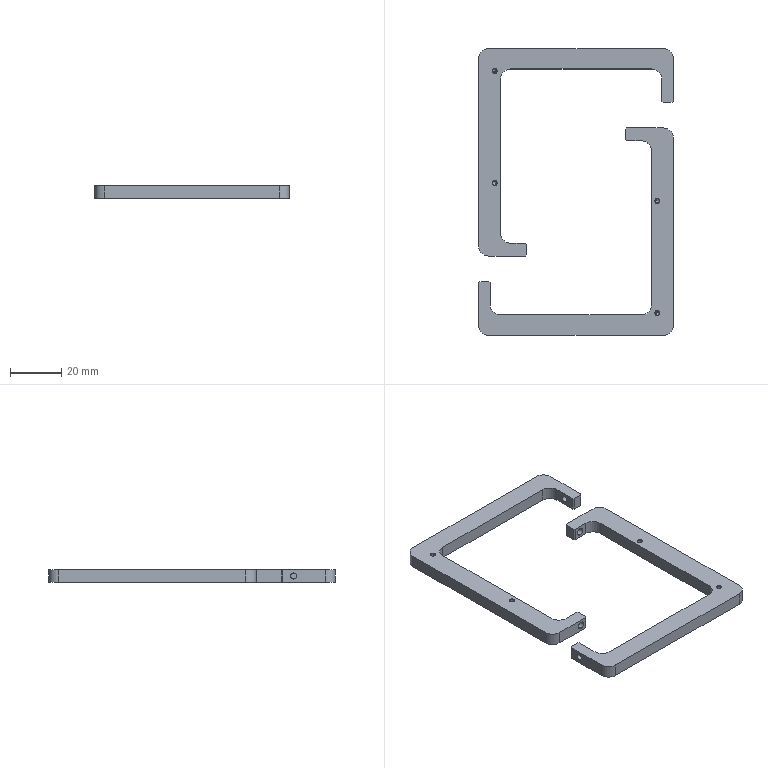CAM job | NX | 3+2 milling, drilling | part box 76 x 112 x 5 mm | stock box 76 x 112 x 5 mm
Tools:
number,name,description,diameter,corner_radius,flute_length,length,flutes
3,CHAMFER_D4-90DEG,倒角D4-90度,4.0,0.0,5.0,50.0,2
5,DRILL_D1.84-11-D3-40,钻刀D1.84-11-D3-40,1.84,0.0,11.0,12.0,2
10,DRILL_D2.4-11-D3-40,钻刀D1.84-11-D3-40,2.4,0.0,11.0,12.0,2
10,DRILL_D2.9-11-D3-40,钻刀D1.84-11-D3-40,2.9,0.0,11.0,12.0,2
6,FORM_M2-12-D3-39,挤压M2-12-D3-39,2.0,0.0,12.5,14.5,2
1,D4_ROUGH,Milling Tool-5 Parameters,4.0,0.0,50.0,75.0,2
2,D4-16-D4-75-3T,D4-16-D4-75-3T,4.0,0.0,16.0,75.0,3
1,CHAMFER_D3-90DEG,倒角D3-90度,3.0,0.0,5.0,50.0,2
Operations:
program,operation,operation_type,tool,method,geometry_group,spindle_rpm,surface_speed,feed_per_tooth,feed_cut,feed_plunge,cut_length_mm,path_length_mm,cut_time_min,machine_time_min
B1,DRILLING_1,Operation,CHAMFER_D4-90DEG,METHOD,WORKPIECE,3000.0,37.0,0.0333,200.0,0.0,16.2,250.449,0.081,0.1044
B2,DRILLING_1_COPY,Operation,DRILL_D1.84-11-D3-40,METHOD,WORKPIECE,3000.0,17.0,0.0167,100.0,0.0,30.4,278.849,0.304,0.3288
B3,DRILLING_1_COPY_COPY,Operation,FORM_M2-12-D3-39,METHOD,WORKPIECE,300.0,1.0,0.2,120.0,0.0,29.2,276.449,0.2433,0.2681
B4,FLOOR_WALL_1,VolumeBased25DMillingOperation,D4_ROUGH,METHOD,WORKPIECE,6500.0,81.0,0.1538,2000.0,100.0,2667.244,2912.294,1.334,1.358
B4,FLOOR_WALL_1_COPY,VolumeBased25DMillingOperation,D4-16-D4-75-3T,METHOD,WORKPIECE,6500.0,81.0,0.041,800.0,100.0,1333.622,1475.488,1.667,1.681
B5,PLANAR_MILL_2,PlanarMilling,D4_ROUGH,METHOD,WORKPIECE,6500.0,81.0,0.1154,1500.0,100.0,10303.227,10451.343,6.869,6.884
B5,PLANAR_MILL_2_COPY,PlanarMilling,D4-16-D4-75-3T,METHOD,WORKPIECE,6500.0,81.0,0.041,800.0,100.0,736.644,887.18,0.9208,0.9359
B6,PLANAR_MILL_1_COPY,PlanarMilling,CHAMFER_D3-90DEG,METHOD,WORKPIECE,6500.0,100.0,0.1178,1200.0,100.0,729.278,888.008,0.6077,0.6236
G55,DRILLING,Operation,CHAMFER_D4-90DEG,METHOD,G55,1200.0,15.0,0.0417,100.0,0.0,4.2,48.4,0.042,0.0464
G55,DRILLING_COPY,Operation,DRILL_D2.4-11-D3-40,METHOD,G55,2000.0,15.0,0.025,100.0,0.0,9.0,58.0,0.09,0.0949
G56,DRILLING_COPY_1,Operation,CHAMFER_D4-90DEG,METHOD,G56,1200.0,15.0,0.0417,100.0,0.0,4.45,48.9,0.0445,0.0489
G56,DRILLING_COPY_COPY,Operation,DRILL_D2.9-11-D3-40,METHOD,G56,2000.0,15.0,0.025,100.0,0.0,9.0,58.0,0.09,0.0949